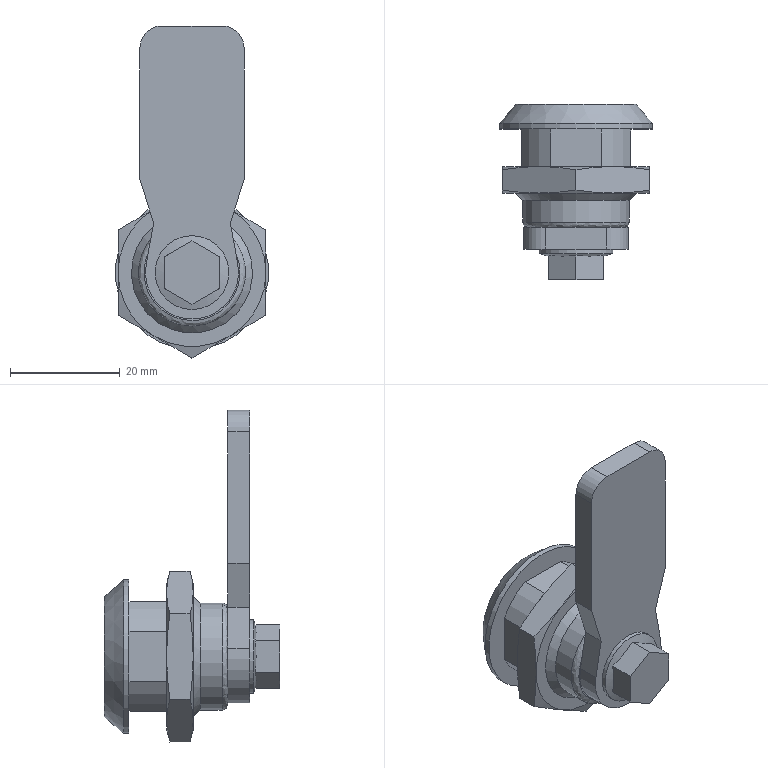Part | STEP file | MS705-18 triangular lock core | 1 solid | 67 faces | box 28 x 32 x 60.591 mm | volume 12821 mm3 | plane 36 | cone 15 | cylinder 14 | spline 2 | commonest cylinder face diameters 22 x4 9.5 x3 8 x2 13.5 x1 16.1 x1 17 x1